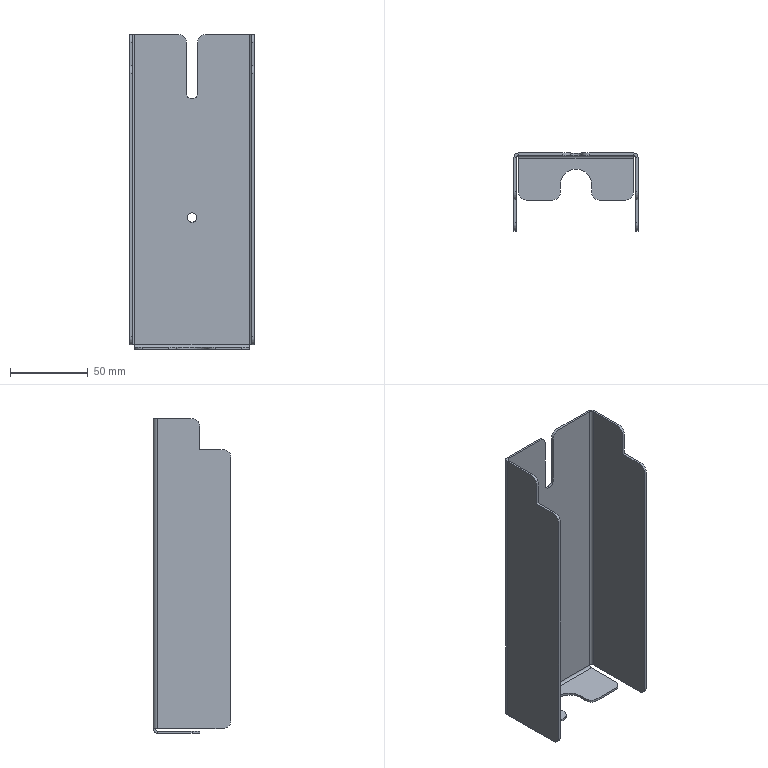Part | NX | features BREP 1 | 1 solid | 55 faces | box 80 x 50 x 203 mm | volume 53607 mm3 | plane 34 | cylinder 21 | commonest cylinder face diameters 10 x12 6 x4 3 x3 7 x1 20 x1
STEP:
#1=CARTESIAN_POINT('',(32.,-30.,-1.5));
#2=VERTEX_POINT('',#1);
#3=CARTESIAN_POINT('',(15.,-30.,-1.5));
#4=VERTEX_POINT('',#3);
#5=CARTESIAN_POINT('',(-37.,-30.,-1.5));
#6=DIRECTION('',(-1.,0.,0.));
#7=VECTOR('',#6,1000.);
#8=LINE('',#5,#7);
#9=EDGE_CURVE('',#2,#4,#8,.T.);
#10=ORIENTED_EDGE('',*,*,#9,.T.);
#11=CARTESIAN_POINT('',(15.,-30.,-3.));
#12=VERTEX_POINT('',#11);
#13=CARTESIAN_POINT('',(15.,-30.,-3.));
#14=DIRECTION('',(0.,0.,-1.));
#15=VECTOR('',#14,1000.);
#16=LINE('',#13,#15);
#17=EDGE_CURVE('',#4,#12,#16,.T.);
#18=ORIENTED_EDGE('',*,*,#17,.T.);
#19=CARTESIAN_POINT('',(32.,-30.,-3.));
#20=VERTEX_POINT('',#19);
#21=CARTESIAN_POINT('',(0.,-30.,-3.));
#22=DIRECTION('',(-1.,0.,0.));
#23=VECTOR('',#22,1000.);
#24=LINE('',#21,#23);
#25=EDGE_CURVE('',#20,#12,#24,.T.);
#26=ORIENTED_EDGE('',*,*,#25,.F.);
#27=CARTESIAN_POINT('',(32.,-30.,-3.));
#28=DIRECTION('',(0.,0.,1.));
#29=VECTOR('',#28,1000.);
#30=LINE('',#27,#29);
#31=EDGE_CURVE('',#20,#2,#30,.T.);
#32=ORIENTED_EDGE('',*,*,#31,.T.);
#33=EDGE_LOOP('',(#10,#18,#26,#32));
#34=FACE_BOUND('',#33,.T.);
#35=CARTESIAN_POINT('',(-37.,-30.,-3.));
#36=DIRECTION('',(0.,1.,0.));
#37=DIRECTION('',(0.,0.,-1.));
#38=AXIS2_PLACEMENT_3D('',#35,#36,#37);
#39=PLANE('',#38);
#40=ADVANCED_FACE('',(#34),#39,.F.);
#41=CARTESIAN_POINT('',(-37.,-1.5,200.));
#42=VERTEX_POINT('',#41);
#43=CARTESIAN_POINT('',(-8.5,-1.5,200.));
#44=VERTEX_POINT('',#43);
#45=CARTESIAN_POINT('',(-40.,-1.5,200.));
#46=DIRECTION('',(1.,0.,0.));
#47=VECTOR('',#46,1000.);
#48=LINE('',#45,#47);
#49=EDGE_CURVE('',#42,#44,#48,.T.);
#50=ORIENTED_EDGE('',*,*,#49,.T.);
#51=CARTESIAN_POINT('',(-8.5,0.,200.));
#52=VERTEX_POINT('',#51);
#53=CARTESIAN_POINT('',(-8.5,0.,200.));
#54=DIRECTION('',(0.,1.,0.));
#55=VECTOR('',#54,1000.);
#56=LINE('',#53,#55);
#57=EDGE_CURVE('',#44,#52,#56,.T.);
#58=ORIENTED_EDGE('',*,*,#57,.T.);
#59=CARTESIAN_POINT('',(-37.,0.,200.));
#60=VERTEX_POINT('',#59);
#61=CARTESIAN_POINT('',(-40.,0.,200.));
#62=DIRECTION('',(1.,0.,0.));
#63=VECTOR('',#62,1000.);
#64=LINE('',#61,#63);
#65=EDGE_CURVE('',#60,#52,#64,.T.);
#66=ORIENTED_EDGE('',*,*,#65,.F.);
#67=CARTESIAN_POINT('',(-37.,0.,200.));
#68=DIRECTION('',(0.,-1.,0.));
#69=VECTOR('',#68,1000.);
#70=LINE('',#67,#69);
#71=EDGE_CURVE('',#60,#42,#70,.T.);
#72=ORIENTED_EDGE('',*,*,#71,.T.);
#73=EDGE_LOOP('',(#50,#58,#66,#72));
#74=FACE_BOUND('',#73,.T.);
#75=CARTESIAN_POINT('',(-38.5,-3.,200.));
#76=DIRECTION('',(0.,0.,1.));
#77=DIRECTION('',(-1.,0.,0.));
#78=AXIS2_PLACEMENT_3D('',#75,#76,#77);
#79=PLANE('',#78);
#80=ADVANCED_FACE('',(#74),#79,.T.);
#81=ORIENTED_EDGE('',*,*,#71,.F.);
#82=CARTESIAN_POINT('',(-40.,-3.,200.));
#83=VERTEX_POINT('',#82);
#84=CARTESIAN_POINT('',(-37.,-3.,200.));
#85=DIRECTION('',(0.,0.,-1.));
#86=DIRECTION('',(1.,0.,0.));
#87=AXIS2_PLACEMENT_3D('',#84,#85,#86);
#88=CIRCLE('',#87,3.);
#89=EDGE_CURVE('',#83,#60,#88,.T.);
#90=ORIENTED_EDGE('',*,*,#89,.F.);
#91=CARTESIAN_POINT('',(-38.5,-3.,200.));
#92=VERTEX_POINT('',#91);
#93=CARTESIAN_POINT('',(-38.5,-3.,200.));
#94=DIRECTION('',(-1.,0.,0.));
#95=VECTOR('',#94,1000.);
#96=LINE('',#93,#95);
#97=EDGE_CURVE('',#92,#83,#96,.T.);
#98=ORIENTED_EDGE('',*,*,#97,.F.);
#99=CARTESIAN_POINT('',(-37.,-3.,200.));
#100=DIRECTION('',(0.,0.,-1.));
#101=DIRECTION('',(1.,0.,0.));
#102=AXIS2_PLACEMENT_3D('',#99,#100,#101);
#103=CIRCLE('',#102,1.5);
#104=EDGE_CURVE('',#92,#42,#103,.T.);
#105=ORIENTED_EDGE('',*,*,#104,.T.);
#106=EDGE_LOOP('',(#81,#90,#98,#105));
#107=FACE_BOUND('',#106,.T.);
#108=CARTESIAN_POINT('',(-37.,0.,200.));
#109=DIRECTION('',(0.,0.,1.));
#110=DIRECTION('',(-1.,0.,0.));
#111=AXIS2_PLACEMENT_3D('',#108,#109,#110);
#112=PLANE('',#111);
#113=ADVANCED_FACE('',(#107),#112,.T.);
#114=CARTESIAN_POINT('',(8.5,0.,200.));
#115=VERTEX_POINT('',#114);
#116=CARTESIAN_POINT('',(37.,0.,200.));
#117=VERTEX_POINT('',#116);
#118=CARTESIAN_POINT('',(-40.,0.,200.));
#119=DIRECTION('',(1.,0.,0.));
#120=VECTOR('',#119,1000.);
#121=LINE('',#118,#120);
#122=EDGE_CURVE('',#115,#117,#121,.T.);
#123=ORIENTED_EDGE('',*,*,#122,.F.);
#124=CARTESIAN_POINT('',(8.5,-1.5,200.));
#125=VERTEX_POINT('',#124);
#126=CARTESIAN_POINT('',(8.5,-1.5,200.));
#127=DIRECTION('',(0.,-1.,0.));
#128=VECTOR('',#127,1000.);
#129=LINE('',#126,#128);
#130=EDGE_CURVE('',#115,#125,#129,.T.);
#131=ORIENTED_EDGE('',*,*,#130,.T.);
#132=CARTESIAN_POINT('',(37.,-1.5,200.));
#133=VERTEX_POINT('',#132);
#134=CARTESIAN_POINT('',(-40.,-1.5,200.));
#135=DIRECTION('',(1.,0.,0.));
#136=VECTOR('',#135,1000.);
#137=LINE('',#134,#136);
#138=EDGE_CURVE('',#125,#133,#137,.T.);
#139=ORIENTED_EDGE('',*,*,#138,.T.);
#140=CARTESIAN_POINT('',(37.,-1.5,200.));
#141=DIRECTION('',(0.,1.,0.));
#142=VECTOR('',#141,1000.);
#143=LINE('',#140,#142);
#144=EDGE_CURVE('',#133,#117,#143,.T.);
#145=ORIENTED_EDGE('',*,*,#144,.T.);
#146=EDGE_LOOP('',(#123,#131,#139,#145));
#147=FACE_BOUND('',#146,.T.);
#148=CARTESIAN_POINT('',(-38.5,-3.,200.));
#149=DIRECTION('',(0.,0.,1.));
#150=DIRECTION('',(-1.,0.,0.));
#151=AXIS2_PLACEMENT_3D('',#148,#149,#150);
#152=PLANE('',#151);
#153=ADVANCED_FACE('',(#147),#152,.T.);
#154=CARTESIAN_POINT('',(-40.,-3.,0.));
#155=VERTEX_POINT('',#154);
#156=CARTESIAN_POINT('',(-38.5,-3.,0.));
#157=VERTEX_POINT('',#156);
#158=CARTESIAN_POINT('',(-40.,-3.,0.));
#159=DIRECTION('',(1.,0.,0.));
#160=VECTOR('',#159,1000.);
#161=LINE('',#158,#160);
#162=EDGE_CURVE('',#155,#157,#161,.T.);
#163=ORIENTED_EDGE('',*,*,#162,.F.);
#164=CARTESIAN_POINT('',(-37.,0.,0.));
#165=VERTEX_POINT('',#164);
#166=CARTESIAN_POINT('',(-37.,-3.,0.));
#167=DIRECTION('',(0.,0.,-1.));
#168=DIRECTION('',(1.,0.,0.));
#169=AXIS2_PLACEMENT_3D('',#166,#167,#168);
#170=CIRCLE('',#169,3.);
#171=EDGE_CURVE('',#155,#165,#170,.T.);
#172=ORIENTED_EDGE('',*,*,#171,.T.);
#173=CARTESIAN_POINT('',(-37.,-1.5,0.));
#174=VERTEX_POINT('',#173);
#175=CARTESIAN_POINT('',(-37.,-1.5,0.));
#176=DIRECTION('',(0.,1.,0.));
#177=VECTOR('',#176,1000.);
#178=LINE('',#175,#177);
#179=EDGE_CURVE('',#174,#165,#178,.T.);
#180=ORIENTED_EDGE('',*,*,#179,.F.);
#181=CARTESIAN_POINT('',(-37.,-3.,0.));
#182=DIRECTION('',(0.,0.,-1.));
#183=DIRECTION('',(1.,0.,0.));
#184=AXIS2_PLACEMENT_3D('',#181,#182,#183);
#185=CIRCLE('',#184,1.5);
#186=EDGE_CURVE('',#157,#174,#185,.T.);
#187=ORIENTED_EDGE('',*,*,#186,.F.);
#188=EDGE_LOOP('',(#163,#172,#180,#187));
#189=FACE_BOUND('',#188,.T.);
#190=CARTESIAN_POINT('',(-40.,-3.,0.));
#191=DIRECTION('',(0.,0.,-1.));
#192=DIRECTION('',(1.,0.,0.));
#193=AXIS2_PLACEMENT_3D('',#190,#191,#192);
#194=PLANE('',#193);
#195=ADVANCED_FACE('',(#189),#194,.T.);
#196=CARTESIAN_POINT('',(-38.5,-45.,0.));
#197=VERTEX_POINT('',#196);
#198=CARTESIAN_POINT('',(-38.5,-50.,0.));
#199=DIRECTION('',(0.,1.,0.));
#200=VECTOR('',#199,1000.);
#201=LINE('',#198,#200);
#202=EDGE_CURVE('',#197,#157,#201,.T.);
#203=ORIENTED_EDGE('',*,*,#202,.F.);
#204=CARTESIAN_POINT('',(-40.,-45.,0.));
#205=VERTEX_POINT('',#204);
#206=CARTESIAN_POINT('',(-37.,-45.,0.));
#207=DIRECTION('',(-1.,0.,0.));
#208=VECTOR('',#207,1000.);
#209=LINE('',#206,#208);
#210=EDGE_CURVE('',#197,#205,#209,.T.);
#211=ORIENTED_EDGE('',*,*,#210,.T.);
#212=CARTESIAN_POINT('',(-40.,-50.,0.));
#213=DIRECTION('',(0.,1.,0.));
#214=VECTOR('',#213,1000.);
#215=LINE('',#212,#214);
#216=EDGE_CURVE('',#205,#155,#215,.T.);
#217=ORIENTED_EDGE('',*,*,#216,.T.);
#218=ORIENTED_EDGE('',*,*,#162,.T.);
#219=EDGE_LOOP('',(#203,#211,#217,#218));
#220=FACE_BOUND('',#219,.T.);
#221=CARTESIAN_POINT('',(-37.,-1.5,0.));
#222=DIRECTION('',(0.,0.,-1.));
#223=DIRECTION('',(1.,0.,0.));
#224=AXIS2_PLACEMENT_3D('',#221,#222,#223);
#225=PLANE('',#224);
#226=ADVANCED_FACE('',(#220),#225,.T.);
#227=CARTESIAN_POINT('',(40.,-3.,200.));
#228=VERTEX_POINT('',#227);
#229=CARTESIAN_POINT('',(38.5,-3.,200.));
#230=VERTEX_POINT('',#229);
#231=CARTESIAN_POINT('',(40.,-3.,200.));
#232=DIRECTION('',(-1.,0.,0.));
#233=VECTOR('',#232,1000.);
#234=LINE('',#231,#233);
#235=EDGE_CURVE('',#228,#230,#234,.T.);
#236=ORIENTED_EDGE('',*,*,#235,.F.);
#237=CARTESIAN_POINT('',(37.,-3.,200.));
#238=DIRECTION('',(0.,0.,-1.));
#239=DIRECTION('',(1.,0.,0.));
#240=AXIS2_PLACEMENT_3D('',#237,#238,#239);
#241=CIRCLE('',#240,3.);
#242=EDGE_CURVE('',#117,#228,#241,.T.);
#243=ORIENTED_EDGE('',*,*,#242,.F.);
#244=ORIENTED_EDGE('',*,*,#144,.F.);
#245=CARTESIAN_POINT('',(37.,-3.,200.));
#246=DIRECTION('',(0.,0.,-1.));
#247=DIRECTION('',(1.,0.,0.));
#248=AXIS2_PLACEMENT_3D('',#245,#246,#247);
#249=CIRCLE('',#248,1.5);
#250=EDGE_CURVE('',#133,#230,#249,.T.);
#251=ORIENTED_EDGE('',*,*,#250,.T.);
#252=EDGE_LOOP('',(#236,#243,#244,#251));
#253=FACE_BOUND('',#252,.T.);
#254=CARTESIAN_POINT('',(40.,-3.,200.));
#255=DIRECTION('',(0.,0.,1.));
#256=DIRECTION('',(-1.,0.,0.));
#257=AXIS2_PLACEMENT_3D('',#254,#255,#256);
#258=PLANE('',#257);
#259=ADVANCED_FACE('',(#253),#258,.T.);
#260=CARTESIAN_POINT('',(38.5,-25.,200.));
#261=VERTEX_POINT('',#260);
#262=CARTESIAN_POINT('',(38.5,0.,200.));
#263=DIRECTION('',(0.,-1.,0.));
#264=VECTOR('',#263,1000.);
#265=LINE('',#262,#264);
#266=EDGE_CURVE('',#230,#261,#265,.T.);
#267=ORIENTED_EDGE('',*,*,#266,.T.);
#268=CARTESIAN_POINT('',(40.,-25.,200.));
#269=VERTEX_POINT('',#268);
#270=CARTESIAN_POINT('',(40.,-25.,200.));
#271=DIRECTION('',(1.,0.,0.));
#272=VECTOR('',#271,1000.);
#273=LINE('',#270,#272);
#274=EDGE_CURVE('',#261,#269,#273,.T.);
#275=ORIENTED_EDGE('',*,*,#274,.T.);
#276=CARTESIAN_POINT('',(40.,0.,200.));
#277=DIRECTION('',(0.,-1.,0.));
#278=VECTOR('',#277,1000.);
#279=LINE('',#276,#278);
#280=EDGE_CURVE('',#228,#269,#279,.T.);
#281=ORIENTED_EDGE('',*,*,#280,.F.);
#282=ORIENTED_EDGE('',*,*,#235,.T.);
#283=EDGE_LOOP('',(#267,#275,#281,#282));
#284=FACE_BOUND('',#283,.T.);
#285=CARTESIAN_POINT('',(37.,-1.5,200.));
#286=DIRECTION('',(0.,0.,1.));
#287=DIRECTION('',(-1.,0.,0.));
#288=AXIS2_PLACEMENT_3D('',#285,#286,#287);
#289=PLANE('',#288);
#290=ADVANCED_FACE('',(#284),#289,.T.);
#291=CARTESIAN_POINT('',(37.,0.,0.));
#292=VERTEX_POINT('',#291);
#293=CARTESIAN_POINT('',(37.,-1.5,0.));
#294=VERTEX_POINT('',#293);
#295=CARTESIAN_POINT('',(37.,0.,0.));
#296=DIRECTION('',(0.,-1.,0.));
#297=VECTOR('',#296,1000.);
#298=LINE('',#295,#297);
#299=EDGE_CURVE('',#292,#294,#298,.T.);
#300=ORIENTED_EDGE('',*,*,#299,.F.);
#301=CARTESIAN_POINT('',(40.,-3.,0.));
#302=VERTEX_POINT('',#301);
#303=CARTESIAN_POINT('',(37.,-3.,0.));
#304=DIRECTION('',(0.,0.,-1.));
#305=DIRECTION('',(1.,0.,0.));
#306=AXIS2_PLACEMENT_3D('',#303,#304,#305);
#307=CIRCLE('',#306,3.);
#308=EDGE_CURVE('',#292,#302,#307,.T.);
#309=ORIENTED_EDGE('',*,*,#308,.T.);
#310=CARTESIAN_POINT('',(38.5,-3.,0.));
#311=VERTEX_POINT('',#310);
#312=CARTESIAN_POINT('',(38.5,-3.,0.));
#313=DIRECTION('',(1.,0.,0.));
#314=VECTOR('',#313,1000.);
#315=LINE('',#312,#314);
#316=EDGE_CURVE('',#311,#302,#315,.T.);
#317=ORIENTED_EDGE('',*,*,#316,.F.);
#318=CARTESIAN_POINT('',(37.,-3.,0.));
#319=DIRECTION('',(0.,0.,-1.));
#320=DIRECTION('',(1.,0.,0.));
#321=AXIS2_PLACEMENT_3D('',#318,#319,#320);
#322=CIRCLE('',#321,1.5);
#323=EDGE_CURVE('',#294,#311,#322,.T.);
#324=ORIENTED_EDGE('',*,*,#323,.F.);
#325=EDGE_LOOP('',(#300,#309,#317,#324));
#326=FACE_BOUND('',#325,.T.);
#327=CARTESIAN_POINT('',(37.,0.,0.));
#328=DIRECTION('',(0.,0.,-1.));
#329=DIRECTION('',(1.,0.,0.));
#330=AXIS2_PLACEMENT_3D('',#327,#328,#329);
#331=PLANE('',#330);
#332=ADVANCED_FACE('',(#326),#331,.T.);
#333=CARTESIAN_POINT('',(38.5,-45.,0.));
#334=VERTEX_POINT('',#333);
#335=CARTESIAN_POINT('',(38.5,0.,0.));
#336=DIRECTION('',(0.,-1.,0.));
#337=VECTOR('',#336,1000.);
#338=LINE('',#335,#337);
#339=EDGE_CURVE('',#311,#334,#338,.T.);
#340=ORIENTED_EDGE('',*,*,#339,.T.);
#341=CARTESIAN_POINT('',(38.5,-50.,5.));
#342=VERTEX_POINT('',#341);
#343=CARTESIAN_POINT('',(38.5,-45.,5.));
#344=DIRECTION('',(-1.,0.,0.));
#345=DIRECTION('',(0.,1.,0.));
#346=AXIS2_PLACEMENT_3D('',#343,#344,#345);
#347=CIRCLE('',#346,5.);
#348=EDGE_CURVE('',#334,#342,#347,.T.);
#349=ORIENTED_EDGE('',*,*,#348,.T.);
#350=CARTESIAN_POINT('',(38.5,-50.,175.));
#351=VERTEX_POINT('',#350);
#352=CARTESIAN_POINT('',(38.5,-50.,200.));
#353=DIRECTION('',(0.,0.,-1.));
#354=VECTOR('',#353,1000.);
#355=LINE('',#352,#354);
#356=EDGE_CURVE('',#351,#342,#355,.T.);
#357=ORIENTED_EDGE('',*,*,#356,.F.);
#358=CARTESIAN_POINT('',(38.5,-45.,180.));
#359=VERTEX_POINT('',#358);
#360=CARTESIAN_POINT('',(38.5,-45.,175.));
#361=DIRECTION('',(-1.,0.,0.));
#362=DIRECTION('',(0.,1.,0.));
#363=AXIS2_PLACEMENT_3D('',#360,#361,#362);
#364=CIRCLE('',#363,5.);
#365=EDGE_CURVE('',#351,#359,#364,.T.);
#366=ORIENTED_EDGE('',*,*,#365,.T.);
#367=CARTESIAN_POINT('',(38.5,-30.,180.));
#368=VERTEX_POINT('',#367);
#369=CARTESIAN_POINT('',(38.5,0.,180.));
#370=DIRECTION('',(0.,1.,0.));
#371=VECTOR('',#370,1000.);
#372=LINE('',#369,#371);
#373=EDGE_CURVE('',#359,#368,#372,.T.);
#374=ORIENTED_EDGE('',*,*,#373,.T.);
#375=CARTESIAN_POINT('',(38.5,-30.,195.));
#376=VERTEX_POINT('',#375);
#377=CARTESIAN_POINT('',(38.5,-30.,200.));
#378=DIRECTION('',(0.,0.,1.));
#379=VECTOR('',#378,1000.);
#380=LINE('',#377,#379);
#381=EDGE_CURVE('',#368,#376,#380,.T.);
#382=ORIENTED_EDGE('',*,*,#381,.T.);
#383=CARTESIAN_POINT('',(38.5,-25.,195.));
#384=DIRECTION('',(-1.,0.,0.));
#385=DIRECTION('',(0.,1.,0.));
#386=AXIS2_PLACEMENT_3D('',#383,#384,#385);
#387=CIRCLE('',#386,5.);
#388=EDGE_CURVE('',#376,#261,#387,.T.);
#389=ORIENTED_EDGE('',*,*,#388,.T.);
#390=ORIENTED_EDGE('',*,*,#266,.F.);
#391=CARTESIAN_POINT('',(38.5,-3.,200.));
#392=DIRECTION('',(0.,0.,-1.));
#393=VECTOR('',#392,1000.);
#394=LINE('',#391,#393);
#395=EDGE_CURVE('',#230,#311,#394,.T.);
#396=ORIENTED_EDGE('',*,*,#395,.T.);
#397=EDGE_LOOP('',(#340,#349,#357,#366,#374,#382,#389,#390,#396));
#398=FACE_BOUND('',#397,.T.);
#399=CARTESIAN_POINT('',(38.5,0.,200.));
#400=DIRECTION('',(1.,0.,0.));
#401=DIRECTION('',(0.,-1.,0.));
#402=AXIS2_PLACEMENT_3D('',#399,#400,#401);
#403=PLANE('',#402);
#404=ADVANCED_FACE('',(#398),#403,.F.);
#405=ORIENTED_EDGE('',*,*,#356,.T.);
#406=CARTESIAN_POINT('',(40.,-50.,5.));
#407=VERTEX_POINT('',#406);
#408=CARTESIAN_POINT('',(40.,-50.,5.));
#409=DIRECTION('',(1.,0.,0.));
#410=VECTOR('',#409,1000.);
#411=LINE('',#408,#410);
#412=EDGE_CURVE('',#342,#407,#411,.T.);
#413=ORIENTED_EDGE('',*,*,#412,.T.);
#414=CARTESIAN_POINT('',(40.,-50.,175.));
#415=VERTEX_POINT('',#414);
#416=CARTESIAN_POINT('',(40.,-50.,200.));
#417=DIRECTION('',(0.,0.,-1.));
#418=VECTOR('',#417,1000.);
#419=LINE('',#416,#418);
#420=EDGE_CURVE('',#415,#407,#419,.T.);
#421=ORIENTED_EDGE('',*,*,#420,.F.);
#422=CARTESIAN_POINT('',(38.5,-50.,175.));
#423=DIRECTION('',(-1.,0.,0.));
#424=VECTOR('',#423,1000.);
#425=LINE('',#422,#424);
#426=EDGE_CURVE('',#415,#351,#425,.T.);
#427=ORIENTED_EDGE('',*,*,#426,.T.);
#428=EDGE_LOOP('',(#405,#413,#421,#427));
#429=FACE_BOUND('',#428,.T.);
#430=CARTESIAN_POINT('',(40.,-50.,200.));
#431=DIRECTION('',(0.,-1.,0.));
#432=DIRECTION('',(0.,0.,1.));
#433=AXIS2_PLACEMENT_3D('',#430,#431,#432);
#434=PLANE('',#433);
#435=ADVANCED_FACE('',(#429),#434,.T.);
#436=ORIENTED_EDGE('',*,*,#420,.T.);
#437=CARTESIAN_POINT('',(40.,-45.,0.));
#438=VERTEX_POINT('',#437);
#439=CARTESIAN_POINT('',(40.,-45.,5.));
#440=DIRECTION('',(1.,0.,0.));
#441=DIRECTION('',(0.,1.,0.));
#442=AXIS2_PLACEMENT_3D('',#439,#440,#441);
#443=CIRCLE('',#442,5.);
#444=EDGE_CURVE('',#407,#438,#443,.T.);
#445=ORIENTED_EDGE('',*,*,#444,.T.);
#446=CARTESIAN_POINT('',(40.,0.,0.));
#447=DIRECTION('',(0.,-1.,0.));
#448=VECTOR('',#447,1000.);
#449=LINE('',#446,#448);
#450=EDGE_CURVE('',#302,#438,#449,.T.);
#451=ORIENTED_EDGE('',*,*,#450,.F.);
#452=CARTESIAN_POINT('',(40.,-3.,200.));
#453=DIRECTION('',(0.,0.,-1.));
#454=VECTOR('',#453,1000.);
#455=LINE('',#452,#454);
#456=EDGE_CURVE('',#228,#302,#455,.T.);
#457=ORIENTED_EDGE('',*,*,#456,.F.);
#458=ORIENTED_EDGE('',*,*,#280,.T.);
#459=CARTESIAN_POINT('',(40.,-30.,195.));
#460=VERTEX_POINT('',#459);
#461=CARTESIAN_POINT('',(40.,-25.,195.));
#462=DIRECTION('',(1.,0.,0.));
#463=DIRECTION('',(0.,1.,0.));
#464=AXIS2_PLACEMENT_3D('',#461,#462,#463);
#465=CIRCLE('',#464,5.);
#466=EDGE_CURVE('',#269,#460,#465,.T.);
#467=ORIENTED_EDGE('',*,*,#466,.T.);
#468=CARTESIAN_POINT('',(40.,-30.,180.));
#469=VERTEX_POINT('',#468);
#470=CARTESIAN_POINT('',(40.,-30.,200.));
#471=DIRECTION('',(0.,0.,1.));
#472=VECTOR('',#471,1000.);
#473=LINE('',#470,#472);
#474=EDGE_CURVE('',#469,#460,#473,.T.);
#475=ORIENTED_EDGE('',*,*,#474,.F.);
#476=CARTESIAN_POINT('',(40.,-45.,180.));
#477=VERTEX_POINT('',#476);
#478=CARTESIAN_POINT('',(40.,-30.,180.));
#479=DIRECTION('',(0.,1.,0.));
#480=VECTOR('',#479,1000.);
#481=LINE('',#478,#480);
#482=EDGE_CURVE('',#477,#469,#481,.T.);
#483=ORIENTED_EDGE('',*,*,#482,.F.);
#484=CARTESIAN_POINT('',(40.,-45.,175.));
#485=DIRECTION('',(1.,0.,0.));
#486=DIRECTION('',(0.,1.,0.));
#487=AXIS2_PLACEMENT_3D('',#484,#485,#486);
#488=CIRCLE('',#487,5.);
#489=EDGE_CURVE('',#477,#415,#488,.T.);
#490=ORIENTED_EDGE('',*,*,#489,.T.);
#491=EDGE_LOOP('',(#436,#445,#451,#457,#458,#467,#475,#483,#490));
#492=FACE_BOUND('',#491,.T.);
#493=CARTESIAN_POINT('',(40.,0.,200.));
#494=DIRECTION('',(1.,0.,0.));
#495=DIRECTION('',(0.,-1.,0.));
#496=AXIS2_PLACEMENT_3D('',#493,#494,#495);
#497=PLANE('',#496);
#498=ADVANCED_FACE('',(#492),#497,.T.);
#499=ORIENTED_EDGE('',*,*,#308,.F.);
#500=CARTESIAN_POINT('',(37.,0.,200.));
#501=DIRECTION('',(0.,0.,-1.));
#502=VECTOR('',#501,1000.);
#503=LINE('',#500,#502);
#504=EDGE_CURVE('',#117,#292,#503,.T.);
#505=ORIENTED_EDGE('',*,*,#504,.F.);
#506=ORIENTED_EDGE('',*,*,#242,.T.);
#507=ORIENTED_EDGE('',*,*,#456,.T.);
#508=EDGE_LOOP('',(#499,#505,#506,#507));
#509=FACE_BOUND('',#508,.T.);
#510=CARTESIAN_POINT('',(37.,-3.,200.));
#511=DIRECTION('',(0.,0.,-1.));
#512=DIRECTION('',(1.,0.,0.));
#513=AXIS2_PLACEMENT_3D('',#510,#511,#512);
#514=CYLINDRICAL_SURFACE('',#513,3.);
#515=ADVANCED_FACE('',(#509),#514,.T.);
#516=CARTESIAN_POINT('',(3.5,0.,195.));
#517=VERTEX_POINT('',#516);
#518=CARTESIAN_POINT('',(3.5,0.,162.));
#519=VERTEX_POINT('',#518);
#520=CARTESIAN_POINT('',(3.5,0.,200.));
#521=DIRECTION('',(0.,0.,-1.));
#522=VECTOR('',#521,1000.);
#523=LINE('',#520,#522);
#524=EDGE_CURVE('',#517,#519,#523,.T.);
#525=ORIENTED_EDGE('',*,*,#524,.F.);
#526=CARTESIAN_POINT('',(8.5,0.,195.));
#527=DIRECTION('',(0.,1.,0.));
#528=DIRECTION('',(-1.,0.,0.));
#529=AXIS2_PLACEMENT_3D('',#526,#527,#528);
#530=CIRCLE('',#529,5.);
#531=EDGE_CURVE('',#517,#115,#530,.T.);
#532=ORIENTED_EDGE('',*,*,#531,.T.);
#533=ORIENTED_EDGE('',*,*,#122,.T.);
#534=ORIENTED_EDGE('',*,*,#504,.T.);
#535=CARTESIAN_POINT('',(-40.,0.,0.));
#536=DIRECTION('',(1.,0.,0.));
#537=VECTOR('',#536,1000.);
#538=LINE('',#535,#537);
#539=EDGE_CURVE('',#165,#292,#538,.T.);
#540=ORIENTED_EDGE('',*,*,#539,.F.);
#541=CARTESIAN_POINT('',(-37.,0.,200.));
#542=DIRECTION('',(0.,0.,-1.));
#543=VECTOR('',#542,1000.);
#544=LINE('',#541,#543);
#545=EDGE_CURVE('',#60,#165,#544,.T.);
#546=ORIENTED_EDGE('',*,*,#545,.F.);
#547=ORIENTED_EDGE('',*,*,#65,.T.);
#548=CARTESIAN_POINT('',(-3.5,0.,195.));
#549=VERTEX_POINT('',#548);
#550=CARTESIAN_POINT('',(-8.5,0.,195.));
#551=DIRECTION('',(0.,1.,0.));
#552=DIRECTION('',(-1.,0.,0.));
#553=AXIS2_PLACEMENT_3D('',#550,#551,#552);
#554=CIRCLE('',#553,5.);
#555=EDGE_CURVE('',#52,#549,#554,.T.);
#556=ORIENTED_EDGE('',*,*,#555,.T.);
#557=CARTESIAN_POINT('',(-3.5,0.,162.));
#558=VERTEX_POINT('',#557);
#559=CARTESIAN_POINT('',(-3.5,0.,200.));
#560=DIRECTION('',(0.,0.,1.));
#561=VECTOR('',#560,1000.);
#562=LINE('',#559,#561);
#563=EDGE_CURVE('',#558,#549,#562,.T.);
#564=ORIENTED_EDGE('',*,*,#563,.F.);
#565=CARTESIAN_POINT('',(0.,0.,162.));
#566=DIRECTION('',(0.,1.,0.));
#567=DIRECTION('',(-1.,0.,0.));
#568=AXIS2_PLACEMENT_3D('',#565,#566,#567);
#569=CIRCLE('',#568,3.5);
#570=EDGE_CURVE('',#519,#558,#569,.T.);
#571=ORIENTED_EDGE('',*,*,#570,.F.);
#572=EDGE_LOOP('',(#525,#532,#533,#534,#540,#546,#547,#556,#564,#571));
#573=FACE_BOUND('',#572,.T.);
#574=CARTESIAN_POINT('',(-3.,0.,82.));
#575=VERTEX_POINT('',#574);
#576=CARTESIAN_POINT('',(0.,0.,82.));
#577=DIRECTION('',(0.,1.,0.));
#578=DIRECTION('',(-1.,0.,0.));
#579=AXIS2_PLACEMENT_3D('',#576,#577,#578);
#580=CIRCLE('',#579,3.);
#581=EDGE_CURVE('',#575,#575,#580,.T.);
#582=ORIENTED_EDGE('',*,*,#581,.F.);
#583=EDGE_LOOP('',(#582));
#584=FACE_BOUND('',#583,.T.);
#585=CARTESIAN_POINT('',(-40.,0.,200.));
#586=DIRECTION('',(0.,1.,0.));
#587=DIRECTION('',(1.,0.,0.));
#588=AXIS2_PLACEMENT_3D('',#585,#586,#587);
#589=PLANE('',#588);
#590=ADVANCED_FACE('',(#573,#584),#589,.T.);
#591=ORIENTED_EDGE('',*,*,#171,.F.);
#592=CARTESIAN_POINT('',(-40.,-3.,200.));
#593=DIRECTION('',(0.,0.,-1.));
#594=VECTOR('',#593,1000.);
#595=LINE('',#592,#594);
#596=EDGE_CURVE('',#83,#155,#595,.T.);
#597=ORIENTED_EDGE('',*,*,#596,.F.);
#598=ORIENTED_EDGE('',*,*,#89,.T.);
#599=ORIENTED_EDGE('',*,*,#545,.T.);
#600=EDGE_LOOP('',(#591,#597,#598,#599));
#601=FACE_BOUND('',#600,.T.);
#602=CARTESIAN_POINT('',(-37.,-3.,200.));
#603=DIRECTION('',(0.,0.,-1.));
#604=DIRECTION('',(1.,0.,0.));
#605=AXIS2_PLACEMENT_3D('',#602,#603,#604);
#606=CYLINDRICAL_SURFACE('',#605,3.);
#607=ADVANCED_FACE('',(#601),#606,.T.);
#608=ORIENTED_EDGE('',*,*,#216,.F.);
#609=CARTESIAN_POINT('',(-40.,-50.,5.));
#610=VERTEX_POINT('',#609);
#611=CARTESIAN_POINT('',(-40.,-45.,5.));
#612=DIRECTION('',(-1.,0.,0.));
#613=DIRECTION('',(0.,0.,1.));
#614=AXIS2_PLACEMENT_3D('',#611,#612,#613);
#615=CIRCLE('',#614,5.);
#616=EDGE_CURVE('',#205,#610,#615,.T.);
#617=ORIENTED_EDGE('',*,*,#616,.T.);
#618=CARTESIAN_POINT('',(-40.,-50.,175.));
#619=VERTEX_POINT('',#618);
#620=CARTESIAN_POINT('',(-40.,-50.,200.));
#621=DIRECTION('',(0.,0.,-1.));
#622=VECTOR('',#621,1000.);
#623=LINE('',#620,#622);
#624=EDGE_CURVE('',#619,#610,#623,.T.);
#625=ORIENTED_EDGE('',*,*,#624,.F.);
#626=CARTESIAN_POINT('',(-40.,-45.,180.));
#627=VERTEX_POINT('',#626);
#628=CARTESIAN_POINT('',(-40.,-45.,175.));
#629=DIRECTION('',(-1.,0.,0.));
#630=DIRECTION('',(0.,0.,1.));
#631=AXIS2_PLACEMENT_3D('',#628,#629,#630);
#632=CIRCLE('',#631,5.);
#633=EDGE_CURVE('',#619,#627,#632,.T.);
#634=ORIENTED_EDGE('',*,*,#633,.T.);
#635=CARTESIAN_POINT('',(-40.,-30.,180.));
#636=VERTEX_POINT('',#635);
#637=CARTESIAN_POINT('',(-40.,-30.,180.));
#638=DIRECTION('',(0.,1.,0.));
#639=VECTOR('',#638,1000.);
#640=LINE('',#637,#639);
#641=EDGE_CURVE('',#627,#636,#640,.T.);
#642=ORIENTED_EDGE('',*,*,#641,.T.);
#643=CARTESIAN_POINT('',(-40.,-30.,195.));
#644=VERTEX_POINT('',#643);
#645=CARTESIAN_POINT('',(-40.,-30.,200.));
#646=DIRECTION('',(0.,0.,1.));
#647=VECTOR('',#646,1000.);
#648=LINE('',#645,#647);
#649=EDGE_CURVE('',#636,#644,#648,.T.);
#650=ORIENTED_EDGE('',*,*,#649,.T.);
#651=CARTESIAN_POINT('',(-40.,-25.,200.));
#652=VERTEX_POINT('',#651);
#653=CARTESIAN_POINT('',(-40.,-25.,195.));
#654=DIRECTION('',(-1.,0.,0.));
#655=DIRECTION('',(0.,0.,1.));
#656=AXIS2_PLACEMENT_3D('',#653,#654,#655);
#657=CIRCLE('',#656,5.);
#658=EDGE_CURVE('',#644,#652,#657,.T.);
#659=ORIENTED_EDGE('',*,*,#658,.T.);
#660=CARTESIAN_POINT('',(-40.,-50.,200.));
#661=DIRECTION('',(0.,1.,0.));
#662=VECTOR('',#661,1000.);
#663=LINE('',#660,#662);
#664=EDGE_CURVE('',#652,#83,#663,.T.);
#665=ORIENTED_EDGE('',*,*,#664,.T.);
#666=ORIENTED_EDGE('',*,*,#596,.T.);
#667=EDGE_LOOP('',(#608,#617,#625,#634,#642,#650,#659,#665,#666));
#668=FACE_BOUND('',#667,.T.);
#669=CARTESIAN_POINT('',(-40.,-50.,200.));
#670=DIRECTION('',(-1.,0.,0.));
#671=DIRECTION('',(0.,0.,-1.));
#672=AXIS2_PLACEMENT_3D('',#669,#670,#671);
#673=PLANE('',#672);
#674=ADVANCED_FACE('',(#668),#673,.T.);
#675=ORIENTED_EDGE('',*,*,#624,.T.);
#676=CARTESIAN_POINT('',(-38.5,-50.,5.));
#677=VERTEX_POINT('',#676);
#678=CARTESIAN_POINT('',(-38.5,-50.,5.));
#679=DIRECTION('',(1.,0.,0.));
#680=VECTOR('',#679,1000.);
#681=LINE('',#678,#680);
#682=EDGE_CURVE('',#610,#677,#681,.T.);
#683=ORIENTED_EDGE('',*,*,#682,.T.);
#684=CARTESIAN_POINT('',(-38.5,-50.,175.));
#685=VERTEX_POINT('',#684);
#686=CARTESIAN_POINT('',(-38.5,-50.,200.));
#687=DIRECTION('',(0.,0.,-1.));
#688=VECTOR('',#687,1000.);
#689=LINE('',#686,#688);
#690=EDGE_CURVE('',#685,#677,#689,.T.);
#691=ORIENTED_EDGE('',*,*,#690,.F.);
#692=CARTESIAN_POINT('',(-40.,-50.,175.));
#693=DIRECTION('',(-1.,0.,0.));
#694=VECTOR('',#693,1000.);
#695=LINE('',#692,#694);
#696=EDGE_CURVE('',#685,#619,#695,.T.);
#697=ORIENTED_EDGE('',*,*,#696,.T.);
#698=EDGE_LOOP('',(#675,#683,#691,#697));
#699=FACE_BOUND('',#698,.T.);
#700=CARTESIAN_POINT('',(-38.5,-50.,200.));
#701=DIRECTION('',(0.,-1.,0.));
#702=DIRECTION('',(0.,0.,1.));
#703=AXIS2_PLACEMENT_3D('',#700,#701,#702);
#704=PLANE('',#703);
#705=ADVANCED_FACE('',(#699),#704,.T.);
#706=ORIENTED_EDGE('',*,*,#690,.T.);
#707=CARTESIAN_POINT('',(-38.5,-45.,5.));
#708=DIRECTION('',(1.,0.,0.));
#709=DIRECTION('',(0.,0.,1.));
#710=AXIS2_PLACEMENT_3D('',#707,#708,#709);
#711=CIRCLE('',#710,5.);
#712=EDGE_CURVE('',#677,#197,#711,.T.);
#713=ORIENTED_EDGE('',*,*,#712,.T.);
#714=ORIENTED_EDGE('',*,*,#202,.T.);
#715=CARTESIAN_POINT('',(-38.5,-3.,200.));
#716=DIRECTION('',(0.,0.,-1.));
#717=VECTOR('',#716,1000.);
#718=LINE('',#715,#717);
#719=EDGE_CURVE('',#92,#157,#718,.T.);
#720=ORIENTED_EDGE('',*,*,#719,.F.);
#721=CARTESIAN_POINT('',(-38.5,-25.,200.));
#722=VERTEX_POINT('',#721);
#723=CARTESIAN_POINT('',(-38.5,-50.,200.));
#724=DIRECTION('',(0.,1.,0.));
#725=VECTOR('',#724,1000.);
#726=LINE('',#723,#725);
#727=EDGE_CURVE('',#722,#92,#726,.T.);
#728=ORIENTED_EDGE('',*,*,#727,.F.);
#729=CARTESIAN_POINT('',(-38.5,-30.,195.));
#730=VERTEX_POINT('',#729);
#731=CARTESIAN_POINT('',(-38.5,-25.,195.));
#732=DIRECTION('',(1.,0.,0.));
#733=DIRECTION('',(0.,0.,1.));
#734=AXIS2_PLACEMENT_3D('',#731,#732,#733);
#735=CIRCLE('',#734,5.);
#736=EDGE_CURVE('',#722,#730,#735,.T.);
#737=ORIENTED_EDGE('',*,*,#736,.T.);
#738=CARTESIAN_POINT('',(-38.5,-30.,180.));
#739=VERTEX_POINT('',#738);
#740=CARTESIAN_POINT('',(-38.5,-30.,200.));
#741=DIRECTION('',(0.,0.,-1.));
#742=VECTOR('',#741,1000.);
#743=LINE('',#740,#742);
#744=EDGE_CURVE('',#730,#739,#743,.T.);
#745=ORIENTED_EDGE('',*,*,#744,.T.);
#746=CARTESIAN_POINT('',(-38.5,-45.,180.));
#747=VERTEX_POINT('',#746);
#748=CARTESIAN_POINT('',(-38.5,-50.,180.));
#749=DIRECTION('',(0.,-1.,0.));
#750=VECTOR('',#749,1000.);
#751=LINE('',#748,#750);
#752=EDGE_CURVE('',#739,#747,#751,.T.);
#753=ORIENTED_EDGE('',*,*,#752,.T.);
#754=CARTESIAN_POINT('',(-38.5,-45.,175.));
#755=DIRECTION('',(1.,0.,0.));
#756=DIRECTION('',(0.,0.,1.));
#757=AXIS2_PLACEMENT_3D('',#754,#755,#756);
#758=CIRCLE('',#757,5.);
#759=EDGE_CURVE('',#747,#685,#758,.T.);
#760=ORIENTED_EDGE('',*,*,#759,.T.);
#761=EDGE_LOOP('',(#706,#713,#714,#720,#728,#737,#745,#753,#760));
#762=FACE_BOUND('',#761,.T.);
#763=CARTESIAN_POINT('',(-38.5,-50.,200.));
#764=DIRECTION('',(-1.,0.,0.));
#765=DIRECTION('',(0.,0.,-1.));
#766=AXIS2_PLACEMENT_3D('',#763,#764,#765);
#767=PLANE('',#766);
#768=ADVANCED_FACE('',(#762),#767,.F.);
#769=ORIENTED_EDGE('',*,*,#186,.T.);
#770=CARTESIAN_POINT('',(-37.,-1.5,200.));
#771=DIRECTION('',(0.,0.,-1.));
#772=VECTOR('',#771,1000.);
#773=LINE('',#770,#772);
#774=EDGE_CURVE('',#42,#174,#773,.T.);
#775=ORIENTED_EDGE('',*,*,#774,.F.);
#776=ORIENTED_EDGE('',*,*,#104,.F.);
#777=ORIENTED_EDGE('',*,*,#719,.T.);
#778=EDGE_LOOP('',(#769,#775,#776,#777));
#779=FACE_BOUND('',#778,.T.);
#780=CARTESIAN_POINT('',(-37.,-3.,200.));
#781=DIRECTION('',(0.,0.,-1.));
#782=DIRECTION('',(1.,0.,0.));
#783=AXIS2_PLACEMENT_3D('',#780,#781,#782);
#784=CYLINDRICAL_SURFACE('',#783,1.5);
#785=ADVANCED_FACE('',(#779),#784,.F.);
#786=CARTESIAN_POINT('',(0.,-1.5,79.));
#787=VERTEX_POINT('',#786);
#788=CARTESIAN_POINT('',(0.,-1.5,82.));
#789=DIRECTION('',(0.,-1.,0.));
#790=DIRECTION('',(0.,0.,-1.));
#791=AXIS2_PLACEMENT_3D('',#788,#789,#790);
#792=CIRCLE('',#791,3.);
#793=EDGE_CURVE('',#787,#787,#792,.T.);
#794=ORIENTED_EDGE('',*,*,#793,.F.);
#795=EDGE_LOOP('',(#794));
#796=FACE_BOUND('',#795,.T.);
#797=ORIENTED_EDGE('',*,*,#138,.F.);
#798=CARTESIAN_POINT('',(3.5,-1.5,195.));
#799=VERTEX_POINT('',#798);
#800=CARTESIAN_POINT('',(8.5,-1.5,195.));
#801=DIRECTION('',(0.,-1.,0.));
#802=DIRECTION('',(-1.,0.,0.));
#803=AXIS2_PLACEMENT_3D('',#800,#801,#802);
#804=CIRCLE('',#803,5.);
#805=EDGE_CURVE('',#125,#799,#804,.T.);
#806=ORIENTED_EDGE('',*,*,#805,.T.);
#807=CARTESIAN_POINT('',(3.5,-1.5,162.));
#808=VERTEX_POINT('',#807);
#809=CARTESIAN_POINT('',(3.5,-1.5,200.));
#810=DIRECTION('',(0.,0.,-1.));
#811=VECTOR('',#810,1000.);
#812=LINE('',#809,#811);
#813=EDGE_CURVE('',#799,#808,#812,.T.);
#814=ORIENTED_EDGE('',*,*,#813,.T.);
#815=CARTESIAN_POINT('',(-3.5,-1.5,162.));
#816=VERTEX_POINT('',#815);
#817=CARTESIAN_POINT('',(0.,-1.5,162.));
#818=DIRECTION('',(0.,1.,0.));
#819=DIRECTION('',(-1.,0.,0.));
#820=AXIS2_PLACEMENT_3D('',#817,#818,#819);
#821=CIRCLE('',#820,3.5);
#822=EDGE_CURVE('',#808,#816,#821,.T.);
#823=ORIENTED_EDGE('',*,*,#822,.T.);
#824=CARTESIAN_POINT('',(-3.5,-1.5,195.));
#825=VERTEX_POINT('',#824);
#826=CARTESIAN_POINT('',(-3.5,-1.5,200.));
#827=DIRECTION('',(0.,0.,1.));
#828=VECTOR('',#827,1000.);
#829=LINE('',#826,#828);
#830=EDGE_CURVE('',#816,#825,#829,.T.);
#831=ORIENTED_EDGE('',*,*,#830,.T.);
#832=CARTESIAN_POINT('',(-8.5,-1.5,195.));
#833=DIRECTION('',(0.,-1.,0.));
#834=DIRECTION('',(-1.,0.,0.));
#835=AXIS2_PLACEMENT_3D('',#832,#833,#834);
#836=CIRCLE('',#835,5.);
#837=EDGE_CURVE('',#825,#44,#836,.T.);
#838=ORIENTED_EDGE('',*,*,#837,.T.);
#839=ORIENTED_EDGE('',*,*,#49,.F.);
#840=ORIENTED_EDGE('',*,*,#774,.T.);
#841=CARTESIAN_POINT('',(-40.,-1.5,0.));
#842=DIRECTION('',(1.,0.,0.));
#843=VECTOR('',#842,1000.);
#844=LINE('',#841,#843);
#845=EDGE_CURVE('',#174,#294,#844,.T.);
#846=ORIENTED_EDGE('',*,*,#845,.T.);
#847=CARTESIAN_POINT('',(37.,-1.5,200.));
#848=DIRECTION('',(0.,0.,-1.));
#849=VECTOR('',#848,1000.);
#850=LINE('',#847,#849);
#851=EDGE_CURVE('',#133,#294,#850,.T.);
#852=ORIENTED_EDGE('',*,*,#851,.F.);
#853=EDGE_LOOP('',(#797,#806,#814,#823,#831,#838,#839,#840,#846,#852));
#854=FACE_BOUND('',#853,.T.);
#855=CARTESIAN_POINT('',(-40.,-1.5,200.));
#856=DIRECTION('',(0.,1.,0.));
#857=DIRECTION('',(1.,0.,0.));
#858=AXIS2_PLACEMENT_3D('',#855,#856,#857);
#859=PLANE('',#858);
#860=ADVANCED_FACE('',(#796,#854),#859,.F.);
#861=ORIENTED_EDGE('',*,*,#323,.T.);
#862=ORIENTED_EDGE('',*,*,#395,.F.);
#863=ORIENTED_EDGE('',*,*,#250,.F.);
#864=ORIENTED_EDGE('',*,*,#851,.T.);
#865=EDGE_LOOP('',(#861,#862,#863,#864));
#866=FACE_BOUND('',#865,.T.);
#867=CARTESIAN_POINT('',(37.,-3.,200.));
#868=DIRECTION('',(0.,0.,-1.));
#869=DIRECTION('',(1.,0.,0.));
#870=AXIS2_PLACEMENT_3D('',#867,#868,#869);
#871=CYLINDRICAL_SURFACE('',#870,1.5);
#872=ADVANCED_FACE('',(#866),#871,.F.);
#873=ORIENTED_EDGE('',*,*,#664,.F.);
#874=CARTESIAN_POINT('',(-38.5,-25.,200.));
#875=DIRECTION('',(1.,0.,0.));
#876=VECTOR('',#875,1000.);
#877=LINE('',#874,#876);
#878=EDGE_CURVE('',#652,#722,#877,.T.);
#879=ORIENTED_EDGE('',*,*,#878,.T.);
#880=ORIENTED_EDGE('',*,*,#727,.T.);
#881=ORIENTED_EDGE('',*,*,#97,.T.);
#882=EDGE_LOOP('',(#873,#879,#880,#881));
#883=FACE_BOUND('',#882,.T.);
#884=CARTESIAN_POINT('',(37.,-3.,200.));
#885=DIRECTION('',(0.,0.,1.));
#886=DIRECTION('',(-1.,0.,0.));
#887=AXIS2_PLACEMENT_3D('',#884,#885,#886);
#888=PLANE('',#887);
#889=ADVANCED_FACE('',(#883),#888,.T.);
#890=ORIENTED_EDGE('',*,*,#450,.T.);
#891=CARTESIAN_POINT('',(38.5,-45.,0.));
#892=DIRECTION('',(-1.,0.,0.));
#893=VECTOR('',#892,1000.);
#894=LINE('',#891,#893);
#895=EDGE_CURVE('',#438,#334,#894,.T.);
#896=ORIENTED_EDGE('',*,*,#895,.T.);
#897=ORIENTED_EDGE('',*,*,#339,.F.);
#898=ORIENTED_EDGE('',*,*,#316,.T.);
#899=EDGE_LOOP('',(#890,#896,#897,#898));
#900=FACE_BOUND('',#899,.T.);
#901=CARTESIAN_POINT('',(37.,-3.,0.));
#902=DIRECTION('',(0.,0.,1.));
#903=DIRECTION('',(-1.,0.,0.));
#904=AXIS2_PLACEMENT_3D('',#901,#902,#903);
#905=PLANE('',#904);
#906=ADVANCED_FACE('',(#900),#905,.F.);
#907=CARTESIAN_POINT('',(-37.,-3.,-1.5));
#908=VERTEX_POINT('',#907);
#909=CARTESIAN_POINT('',(-37.,-3.,-3.));
#910=VERTEX_POINT('',#909);
#911=CARTESIAN_POINT('',(-37.,-3.,-3.));
#912=DIRECTION('',(0.,0.,-1.));
#913=VECTOR('',#912,1000.);
#914=LINE('',#911,#913);
#915=EDGE_CURVE('',#908,#910,#914,.T.);
#916=ORIENTED_EDGE('',*,*,#915,.F.);
#917=CARTESIAN_POINT('',(-37.,-3.,0.));
#918=DIRECTION('',(-1.,0.,0.));
#919=DIRECTION('',(0.,1.,0.));
#920=AXIS2_PLACEMENT_3D('',#917,#918,#919);
#921=CIRCLE('',#920,1.5);
#922=EDGE_CURVE('',#174,#908,#921,.T.);
#923=ORIENTED_EDGE('',*,*,#922,.F.);
#924=ORIENTED_EDGE('',*,*,#179,.T.);
#925=CARTESIAN_POINT('',(-37.,-3.,0.));
#926=DIRECTION('',(-1.,0.,0.));
#927=DIRECTION('',(0.,1.,0.));
#928=AXIS2_PLACEMENT_3D('',#925,#926,#927);
#929=CIRCLE('',#928,3.);
#930=EDGE_CURVE('',#165,#910,#929,.T.);
#931=ORIENTED_EDGE('',*,*,#930,.T.);
#932=EDGE_LOOP('',(#916,#923,#924,#931));
#933=FACE_BOUND('',#932,.T.);
#934=CARTESIAN_POINT('',(-37.,-3.,0.));
#935=DIRECTION('',(-1.,0.,0.));
#936=DIRECTION('',(0.,1.,0.));
#937=AXIS2_PLACEMENT_3D('',#934,#935,#936);
#938=PLANE('',#937);
#939=ADVANCED_FACE('',(#933),#938,.T.);
#940=CARTESIAN_POINT('',(37.,-3.,-1.5));
#941=VERTEX_POINT('',#940);
#942=CARTESIAN_POINT('',(37.,-3.,0.));
#943=DIRECTION('',(1.,0.,0.));
#944=DIRECTION('',(0.,1.,0.));
#945=AXIS2_PLACEMENT_3D('',#942,#943,#944);
#946=CIRCLE('',#945,1.5);
#947=EDGE_CURVE('',#941,#294,#946,.T.);
#948=ORIENTED_EDGE('',*,*,#947,.F.);
#949=CARTESIAN_POINT('',(37.,-3.,-3.));
#950=VERTEX_POINT('',#949);
#951=CARTESIAN_POINT('',(37.,-3.,-1.5));
#952=DIRECTION('',(0.,0.,-1.));
#953=VECTOR('',#952,1000.);
#954=LINE('',#951,#953);
#955=EDGE_CURVE('',#941,#950,#954,.T.);
#956=ORIENTED_EDGE('',*,*,#955,.T.);
#957=CARTESIAN_POINT('',(37.,-3.,0.));
#958=DIRECTION('',(1.,0.,0.));
#959=DIRECTION('',(0.,1.,0.));
#960=AXIS2_PLACEMENT_3D('',#957,#958,#959);
#961=CIRCLE('',#960,3.);
#962=EDGE_CURVE('',#950,#292,#961,.T.);
#963=ORIENTED_EDGE('',*,*,#962,.T.);
#964=ORIENTED_EDGE('',*,*,#299,.T.);
#965=EDGE_LOOP('',(#948,#956,#963,#964));
#966=FACE_BOUND('',#965,.T.);
#967=CARTESIAN_POINT('',(37.,-3.,0.));
#968=DIRECTION('',(-1.,0.,0.));
#969=DIRECTION('',(0.,1.,0.));
#970=AXIS2_PLACEMENT_3D('',#967,#968,#969);
#971=PLANE('',#970);
#972=ADVANCED_FACE('',(#966),#971,.F.);
#973=ORIENTED_EDGE('',*,*,#539,.T.);
#974=ORIENTED_EDGE('',*,*,#962,.F.);
#975=CARTESIAN_POINT('',(-37.,-3.,-3.));
#976=DIRECTION('',(-1.,0.,0.));
#977=VECTOR('',#976,1000.);
#978=LINE('',#975,#977);
#979=EDGE_CURVE('',#950,#910,#978,.T.);
#980=ORIENTED_EDGE('',*,*,#979,.T.);
#981=ORIENTED_EDGE('',*,*,#930,.F.);
#982=EDGE_LOOP('',(#973,#974,#980,#981));
#983=FACE_BOUND('',#982,.T.);
#984=CARTESIAN_POINT('',(37.,-3.,0.));
#985=DIRECTION('',(1.,0.,0.));
#986=DIRECTION('',(0.,0.,1.));
#987=AXIS2_PLACEMENT_3D('',#984,#985,#986);
#988=CYLINDRICAL_SURFACE('',#987,3.);
#989=ADVANCED_FACE('',(#983),#988,.T.);
#990=ORIENTED_EDGE('',*,*,#845,.F.);
#991=ORIENTED_EDGE('',*,*,#922,.T.);
#992=CARTESIAN_POINT('',(-37.,-3.,-1.5));
#993=DIRECTION('',(1.,0.,0.));
#994=VECTOR('',#993,1000.);
#995=LINE('',#992,#994);
#996=EDGE_CURVE('',#908,#941,#995,.T.);
#997=ORIENTED_EDGE('',*,*,#996,.T.);
#998=ORIENTED_EDGE('',*,*,#947,.T.);
#999=EDGE_LOOP('',(#990,#991,#997,#998));
#1000=FACE_BOUND('',#999,.T.);
#1001=CARTESIAN_POINT('',(37.,-3.,0.));
#1002=DIRECTION('',(1.,0.,0.));
#1003=DIRECTION('',(0.,0.,1.));
#1004=AXIS2_PLACEMENT_3D('',#1001,#1002,#1003);
#1005=CYLINDRICAL_SURFACE('',#1004,1.5);
#1006=ADVANCED_FACE('',(#1000),#1005,.F.);
#1007=CARTESIAN_POINT('',(-37.,-25.,-3.));
#1008=VERTEX_POINT('',#1007);
#1009=CARTESIAN_POINT('',(-37.,0.,-3.));
#1010=DIRECTION('',(0.,1.,0.));
#1011=VECTOR('',#1010,1000.);
#1012=LINE('',#1009,#1011);
#1013=EDGE_CURVE('',#1008,#910,#1012,.T.);
#1014=ORIENTED_EDGE('',*,*,#1013,.F.);
#1015=CARTESIAN_POINT('',(-37.,-25.,-1.5));
#1016=VERTEX_POINT('',#1015);
#1017=CARTESIAN_POINT('',(-37.,-25.,-3.));
#1018=DIRECTION('',(0.,0.,1.));
#1019=VECTOR('',#1018,1000.);
#1020=LINE('',#1017,#1019);
#1021=EDGE_CURVE('',#1008,#1016,#1020,.T.);
#1022=ORIENTED_EDGE('',*,*,#1021,.T.);
#1023=CARTESIAN_POINT('',(-37.,-1.5,-1.5));
#1024=DIRECTION('',(0.,1.,0.));
#1025=VECTOR('',#1024,1000.);
#1026=LINE('',#1023,#1025);
#1027=EDGE_CURVE('',#1016,#908,#1026,.T.);
#1028=ORIENTED_EDGE('',*,*,#1027,.T.);
#1029=ORIENTED_EDGE('',*,*,#915,.T.);
#1030=EDGE_LOOP('',(#1014,#1022,#1028,#1029));
#1031=FACE_BOUND('',#1030,.T.);
#1032=CARTESIAN_POINT('',(-37.,-1.5,-3.));
#1033=DIRECTION('',(1.,0.,0.));
#1034=DIRECTION('',(0.,-1.,0.));
#1035=AXIS2_PLACEMENT_3D('',#1032,#1033,#1034);
#1036=PLANE('',#1035);
#1037=ADVANCED_FACE('',(#1031),#1036,.F.);
#1038=CARTESIAN_POINT('',(37.,-25.,-1.5));
#1039=VERTEX_POINT('',#1038);
#1040=CARTESIAN_POINT('',(37.,-30.,-1.5));
#1041=DIRECTION('',(0.,-1.,0.));
#1042=VECTOR('',#1041,1000.);
#1043=LINE('',#1040,#1042);
#1044=EDGE_CURVE('',#941,#1039,#1043,.T.);
#1045=ORIENTED_EDGE('',*,*,#1044,.T.);
#1046=CARTESIAN_POINT('',(37.,-25.,-3.));
#1047=VERTEX_POINT('',#1046);
#1048=CARTESIAN_POINT('',(37.,-25.,-3.));
#1049=DIRECTION('',(0.,0.,-1.));
#1050=VECTOR('',#1049,1000.);
#1051=LINE('',#1048,#1050);
#1052=EDGE_CURVE('',#1039,#1047,#1051,.T.);
#1053=ORIENTED_EDGE('',*,*,#1052,.T.);
#1054=CARTESIAN_POINT('',(37.,0.,-3.));
#1055=DIRECTION('',(0.,-1.,0.));
#1056=VECTOR('',#1055,1000.);
#1057=LINE('',#1054,#1056);
#1058=EDGE_CURVE('',#950,#1047,#1057,.T.);
#1059=ORIENTED_EDGE('',*,*,#1058,.F.);
#1060=ORIENTED_EDGE('',*,*,#955,.F.);
#1061=EDGE_LOOP('',(#1045,#1053,#1059,#1060));
#1062=FACE_BOUND('',#1061,.T.);
#1063=CARTESIAN_POINT('',(37.,-30.,-3.));
#1064=DIRECTION('',(-1.,0.,0.));
#1065=DIRECTION('',(0.,1.,0.));
#1066=AXIS2_PLACEMENT_3D('',#1063,#1064,#1065);
#1067=PLANE('',#1066);
#1068=ADVANCED_FACE('',(#1062),#1067,.F.);
#1069=CARTESIAN_POINT('',(-10.,-25.,-3.));
#1070=VERTEX_POINT('',#1069);
#1071=CARTESIAN_POINT('',(-10.,-20.,-3.));
#1072=VERTEX_POINT('',#1071);
#1073=CARTESIAN_POINT('',(-10.,-30.,-3.));
#1074=DIRECTION('',(0.,1.,0.));
#1075=VECTOR('',#1074,1000.);
#1076=LINE('',#1073,#1075);
#1077=EDGE_CURVE('',#1070,#1072,#1076,.T.);
#1078=ORIENTED_EDGE('',*,*,#1077,.F.);
#1079=CARTESIAN_POINT('',(-15.,-30.,-3.));
#1080=VERTEX_POINT('',#1079);
#1081=CARTESIAN_POINT('',(-15.,-25.,-3.));
#1082=DIRECTION('',(0.,0.,-1.));
#1083=DIRECTION('',(0.,-1.,0.));
#1084=AXIS2_PLACEMENT_3D('',#1081,#1082,#1083);
#1085=CIRCLE('',#1084,5.);
#1086=EDGE_CURVE('',#1070,#1080,#1085,.T.);
#1087=ORIENTED_EDGE('',*,*,#1086,.T.);
#1088=CARTESIAN_POINT('',(-32.,-30.,-3.));
#1089=VERTEX_POINT('',#1088);
#1090=CARTESIAN_POINT('',(0.,-30.,-3.));
#1091=DIRECTION('',(-1.,0.,0.));
#1092=VECTOR('',#1091,1000.);
#1093=LINE('',#1090,#1092);
#1094=EDGE_CURVE('',#1080,#1089,#1093,.T.);
#1095=ORIENTED_EDGE('',*,*,#1094,.T.);
#1096=CARTESIAN_POINT('',(-32.,-25.,-3.));
#1097=DIRECTION('',(0.,0.,-1.));
#1098=DIRECTION('',(0.,-1.,0.));
#1099=AXIS2_PLACEMENT_3D('',#1096,#1097,#1098);
#1100=CIRCLE('',#1099,5.);
#1101=EDGE_CURVE('',#1089,#1008,#1100,.T.);
#1102=ORIENTED_EDGE('',*,*,#1101,.T.);
#1103=ORIENTED_EDGE('',*,*,#1013,.T.);
#1104=ORIENTED_EDGE('',*,*,#979,.F.);
#1105=ORIENTED_EDGE('',*,*,#1058,.T.);
#1106=CARTESIAN_POINT('',(32.,-25.,-3.));
#1107=DIRECTION('',(0.,0.,-1.));
#1108=DIRECTION('',(0.,-1.,0.));
#1109=AXIS2_PLACEMENT_3D('',#1106,#1107,#1108);
#1110=CIRCLE('',#1109,5.);
#1111=EDGE_CURVE('',#1047,#20,#1110,.T.);
#1112=ORIENTED_EDGE('',*,*,#1111,.T.);
#1113=ORIENTED_EDGE('',*,*,#25,.T.);
#1114=CARTESIAN_POINT('',(10.,-25.,-3.));
#1115=VERTEX_POINT('',#1114);
#1116=CARTESIAN_POINT('',(15.,-25.,-3.));
#1117=DIRECTION('',(0.,0.,-1.));
#1118=DIRECTION('',(0.,-1.,0.));
#1119=AXIS2_PLACEMENT_3D('',#1116,#1117,#1118);
#1120=CIRCLE('',#1119,5.);
#1121=EDGE_CURVE('',#12,#1115,#1120,.T.);
#1122=ORIENTED_EDGE('',*,*,#1121,.T.);
#1123=CARTESIAN_POINT('',(10.,-20.,-3.));
#1124=VERTEX_POINT('',#1123);
#1125=CARTESIAN_POINT('',(10.,-30.,-3.));
#1126=DIRECTION('',(0.,-1.,0.));
#1127=VECTOR('',#1126,1000.);
#1128=LINE('',#1125,#1127);
#1129=EDGE_CURVE('',#1124,#1115,#1128,.T.);
#1130=ORIENTED_EDGE('',*,*,#1129,.F.);
#1131=CARTESIAN_POINT('',(0.,-20.,-3.));
#1132=DIRECTION('',(0.,0.,-1.));
#1133=DIRECTION('',(0.,1.,0.));
#1134=AXIS2_PLACEMENT_3D('',#1131,#1132,#1133);
#1135=CIRCLE('',#1134,10.);
#1136=EDGE_CURVE('',#1072,#1124,#1135,.T.);
#1137=ORIENTED_EDGE('',*,*,#1136,.F.);
#1138=EDGE_LOOP('',(#1078,#1087,#1095,#1102,#1103,#1104,#1105,#1112,#1113,#1122,#1130,#1137));
#1139=FACE_BOUND('',#1138,.T.);
#1140=CARTESIAN_POINT('',(0.,0.,-3.));
#1141=DIRECTION('',(0.,0.,1.));
#1142=DIRECTION('',(0.,1.,0.));
#1143=AXIS2_PLACEMENT_3D('',#1140,#1141,#1142);
#1144=PLANE('',#1143);
#1145=ADVANCED_FACE('',(#1139),#1144,.F.);
#1146=CARTESIAN_POINT('',(-15.,-30.,-1.5));
#1147=VERTEX_POINT('',#1146);
#1148=CARTESIAN_POINT('',(-32.,-30.,-1.5));
#1149=VERTEX_POINT('',#1148);
#1150=CARTESIAN_POINT('',(-37.,-30.,-1.5));
#1151=DIRECTION('',(-1.,0.,0.));
#1152=VECTOR('',#1151,1000.);
#1153=LINE('',#1150,#1152);
#1154=EDGE_CURVE('',#1147,#1149,#1153,.T.);
#1155=ORIENTED_EDGE('',*,*,#1154,.F.);
#1156=CARTESIAN_POINT('',(-10.,-25.,-1.5));
#1157=VERTEX_POINT('',#1156);
#1158=CARTESIAN_POINT('',(-15.,-25.,-1.5));
#1159=DIRECTION('',(0.,0.,1.));
#1160=DIRECTION('',(0.,-1.,0.));
#1161=AXIS2_PLACEMENT_3D('',#1158,#1159,#1160);
#1162=CIRCLE('',#1161,5.);
#1163=EDGE_CURVE('',#1147,#1157,#1162,.T.);
#1164=ORIENTED_EDGE('',*,*,#1163,.T.);
#1165=CARTESIAN_POINT('',(-10.,-20.,-1.5));
#1166=VERTEX_POINT('',#1165);
#1167=CARTESIAN_POINT('',(-10.,0.,-1.5));
#1168=DIRECTION('',(0.,-1.,0.));
#1169=VECTOR('',#1168,1000.);
#1170=LINE('',#1167,#1169);
#1171=EDGE_CURVE('',#1166,#1157,#1170,.T.);
#1172=ORIENTED_EDGE('',*,*,#1171,.F.);
#1173=CARTESIAN_POINT('',(10.,-20.,-1.5));
#1174=VERTEX_POINT('',#1173);
#1175=CARTESIAN_POINT('',(0.,-20.,-1.5));
#1176=DIRECTION('',(0.,0.,1.));
#1177=DIRECTION('',(0.,-1.,0.));
#1178=AXIS2_PLACEMENT_3D('',#1175,#1176,#1177);
#1179=CIRCLE('',#1178,10.);
#1180=EDGE_CURVE('',#1174,#1166,#1179,.T.);
#1181=ORIENTED_EDGE('',*,*,#1180,.F.);
#1182=CARTESIAN_POINT('',(10.,-25.,-1.5));
#1183=VERTEX_POINT('',#1182);
#1184=CARTESIAN_POINT('',(10.,0.,-1.5));
#1185=DIRECTION('',(0.,1.,0.));
#1186=VECTOR('',#1185,1000.);
#1187=LINE('',#1184,#1186);
#1188=EDGE_CURVE('',#1183,#1174,#1187,.T.);
#1189=ORIENTED_EDGE('',*,*,#1188,.F.);
#1190=CARTESIAN_POINT('',(15.,-25.,-1.5));
#1191=DIRECTION('',(0.,0.,1.));
#1192=DIRECTION('',(0.,-1.,0.));
#1193=AXIS2_PLACEMENT_3D('',#1190,#1191,#1192);
#1194=CIRCLE('',#1193,5.);
#1195=EDGE_CURVE('',#1183,#4,#1194,.T.);
#1196=ORIENTED_EDGE('',*,*,#1195,.T.);
#1197=ORIENTED_EDGE('',*,*,#9,.F.);
#1198=CARTESIAN_POINT('',(32.,-25.,-1.5));
#1199=DIRECTION('',(0.,0.,1.));
#1200=DIRECTION('',(0.,-1.,0.));
#1201=AXIS2_PLACEMENT_3D('',#1198,#1199,#1200);
#1202=CIRCLE('',#1201,5.);
#1203=EDGE_CURVE('',#2,#1039,#1202,.T.);
#1204=ORIENTED_EDGE('',*,*,#1203,.T.);
#1205=ORIENTED_EDGE('',*,*,#1044,.F.);
#1206=ORIENTED_EDGE('',*,*,#996,.F.);
#1207=ORIENTED_EDGE('',*,*,#1027,.F.);
#1208=CARTESIAN_POINT('',(-32.,-25.,-1.5));
#1209=DIRECTION('',(0.,0.,1.));
#1210=DIRECTION('',(0.,-1.,0.));
#1211=AXIS2_PLACEMENT_3D('',#1208,#1209,#1210);
#1212=CIRCLE('',#1211,5.);
#1213=EDGE_CURVE('',#1016,#1149,#1212,.T.);
#1214=ORIENTED_EDGE('',*,*,#1213,.T.);
#1215=EDGE_LOOP('',(#1155,#1164,#1172,#1181,#1189,#1196,#1197,#1204,#1205,#1206,#1207,#1214));
#1216=FACE_BOUND('',#1215,.T.);
#1217=CARTESIAN_POINT('',(0.,0.,-1.5));
#1218=DIRECTION('',(0.,0.,1.));
#1219=DIRECTION('',(0.,1.,0.));
#1220=AXIS2_PLACEMENT_3D('',#1217,#1218,#1219);
#1221=PLANE('',#1220);
#1222=ADVANCED_FACE('',(#1216),#1221,.T.);
#1223=ORIENTED_EDGE('',*,*,#1094,.F.);
#1224=CARTESIAN_POINT('',(-15.,-30.,-3.));
#1225=DIRECTION('',(0.,0.,1.));
#1226=VECTOR('',#1225,1000.);
#1227=LINE('',#1224,#1226);
#1228=EDGE_CURVE('',#1080,#1147,#1227,.T.);
#1229=ORIENTED_EDGE('',*,*,#1228,.T.);
#1230=ORIENTED_EDGE('',*,*,#1154,.T.);
#1231=CARTESIAN_POINT('',(-32.,-30.,-3.));
#1232=DIRECTION('',(0.,0.,-1.));
#1233=VECTOR('',#1232,1000.);
#1234=LINE('',#1231,#1233);
#1235=EDGE_CURVE('',#1149,#1089,#1234,.T.);
#1236=ORIENTED_EDGE('',*,*,#1235,.T.);
#1237=EDGE_LOOP('',(#1223,#1229,#1230,#1236));
#1238=FACE_BOUND('',#1237,.T.);
#1239=CARTESIAN_POINT('',(-37.,-30.,-3.));
#1240=DIRECTION('',(0.,1.,0.));
#1241=DIRECTION('',(0.,0.,-1.));
#1242=AXIS2_PLACEMENT_3D('',#1239,#1240,#1241);
#1243=PLANE('',#1242);
#1244=ADVANCED_FACE('',(#1238),#1243,.F.);
#1245=ORIENTED_EDGE('',*,*,#744,.F.);
#1246=CARTESIAN_POINT('',(-40.,-30.,195.));
#1247=DIRECTION('',(-1.,0.,0.));
#1248=VECTOR('',#1247,1000.);
#1249=LINE('',#1246,#1248);
#1250=EDGE_CURVE('',#730,#644,#1249,.T.);
#1251=ORIENTED_EDGE('',*,*,#1250,.T.);
#1252=ORIENTED_EDGE('',*,*,#649,.F.);
#1253=CARTESIAN_POINT('',(-40.,-30.,180.));
#1254=DIRECTION('',(1.,0.,0.));
#1255=VECTOR('',#1254,1000.);
#1256=LINE('',#1253,#1255);
#1257=EDGE_CURVE('',#636,#739,#1256,.T.);
#1258=ORIENTED_EDGE('',*,*,#1257,.T.);
#1259=EDGE_LOOP('',(#1245,#1251,#1252,#1258));
#1260=FACE_BOUND('',#1259,.T.);
#1261=CARTESIAN_POINT('',(-40.,-30.,200.));
#1262=DIRECTION('',(0.,1.,0.));
#1263=DIRECTION('',(1.,0.,0.));
#1264=AXIS2_PLACEMENT_3D('',#1261,#1262,#1263);
#1265=PLANE('',#1264);
#1266=ADVANCED_FACE('',(#1260),#1265,.F.);
#1267=ORIENTED_EDGE('',*,*,#641,.F.);
#1268=CARTESIAN_POINT('',(-38.5,-45.,180.));
#1269=DIRECTION('',(1.,0.,0.));
#1270=VECTOR('',#1269,1000.);
#1271=LINE('',#1268,#1270);
#1272=EDGE_CURVE('',#627,#747,#1271,.T.);
#1273=ORIENTED_EDGE('',*,*,#1272,.T.);
#1274=ORIENTED_EDGE('',*,*,#752,.F.);
#1275=ORIENTED_EDGE('',*,*,#1257,.F.);
#1276=EDGE_LOOP('',(#1267,#1273,#1274,#1275));
#1277=FACE_BOUND('',#1276,.T.);
#1278=CARTESIAN_POINT('',(-40.,-30.,180.));
#1279=DIRECTION('',(0.,0.,-1.));
#1280=DIRECTION('',(1.,0.,0.));
#1281=AXIS2_PLACEMENT_3D('',#1278,#1279,#1280);
#1282=PLANE('',#1281);
#1283=ADVANCED_FACE('',(#1277),#1282,.F.);
#1284=ORIENTED_EDGE('',*,*,#373,.F.);
#1285=CARTESIAN_POINT('',(40.,-45.,180.));
#1286=DIRECTION('',(1.,0.,0.));
#1287=VECTOR('',#1286,1000.);
#1288=LINE('',#1285,#1287);
#1289=EDGE_CURVE('',#359,#477,#1288,.T.);
#1290=ORIENTED_EDGE('',*,*,#1289,.T.);
#1291=ORIENTED_EDGE('',*,*,#482,.T.);
#1292=CARTESIAN_POINT('',(-40.,-30.,180.));
#1293=DIRECTION('',(1.,0.,0.));
#1294=VECTOR('',#1293,1000.);
#1295=LINE('',#1292,#1294);
#1296=EDGE_CURVE('',#368,#469,#1295,.T.);
#1297=ORIENTED_EDGE('',*,*,#1296,.F.);
#1298=EDGE_LOOP('',(#1284,#1290,#1291,#1297));
#1299=FACE_BOUND('',#1298,.T.);
#1300=CARTESIAN_POINT('',(-40.,-30.,180.));
#1301=DIRECTION('',(0.,0.,-1.));
#1302=DIRECTION('',(1.,0.,0.));
#1303=AXIS2_PLACEMENT_3D('',#1300,#1301,#1302);
#1304=PLANE('',#1303);
#1305=ADVANCED_FACE('',(#1299),#1304,.F.);
#1306=ORIENTED_EDGE('',*,*,#474,.T.);
#1307=CARTESIAN_POINT('',(38.5,-30.,195.));
#1308=DIRECTION('',(-1.,0.,0.));
#1309=VECTOR('',#1308,1000.);
#1310=LINE('',#1307,#1309);
#1311=EDGE_CURVE('',#460,#376,#1310,.T.);
#1312=ORIENTED_EDGE('',*,*,#1311,.T.);
#1313=ORIENTED_EDGE('',*,*,#381,.F.);
#1314=ORIENTED_EDGE('',*,*,#1296,.T.);
#1315=EDGE_LOOP('',(#1306,#1312,#1313,#1314));
#1316=FACE_BOUND('',#1315,.T.);
#1317=CARTESIAN_POINT('',(-40.,-30.,200.));
#1318=DIRECTION('',(0.,1.,0.));
#1319=DIRECTION('',(1.,0.,0.));
#1320=AXIS2_PLACEMENT_3D('',#1317,#1318,#1319);
#1321=PLANE('',#1320);
#1322=ADVANCED_FACE('',(#1316),#1321,.F.);
#1323=ORIENTED_EDGE('',*,*,#581,.T.);
#1324=EDGE_LOOP('',(#1323));
#1325=FACE_BOUND('',#1324,.T.);
#1326=ORIENTED_EDGE('',*,*,#793,.T.);
#1327=EDGE_LOOP('',(#1326));
#1328=FACE_BOUND('',#1327,.T.);
#1329=CARTESIAN_POINT('',(0.,-1.5,82.));
#1330=DIRECTION('',(0.,-1.,0.));
#1331=DIRECTION('',(0.,0.,1.));
#1332=AXIS2_PLACEMENT_3D('',#1329,#1330,#1331);
#1333=CYLINDRICAL_SURFACE('',#1332,3.);
#1334=ADVANCED_FACE('',(#1325,#1328),#1333,.F.);
#1335=ORIENTED_EDGE('',*,*,#563,.T.);
#1336=CARTESIAN_POINT('',(-3.5,-1.5,195.));
#1337=DIRECTION('',(0.,-1.,0.));
#1338=VECTOR('',#1337,1000.);
#1339=LINE('',#1336,#1338);
#1340=EDGE_CURVE('',#549,#825,#1339,.T.);
#1341=ORIENTED_EDGE('',*,*,#1340,.T.);
#1342=ORIENTED_EDGE('',*,*,#830,.F.);
#1343=CARTESIAN_POINT('',(-3.5,-10.,162.));
#1344=DIRECTION('',(0.,1.,0.));
#1345=VECTOR('',#1344,1000.);
#1346=LINE('',#1343,#1345);
#1347=EDGE_CURVE('',#816,#558,#1346,.T.);
#1348=ORIENTED_EDGE('',*,*,#1347,.T.);
#1349=EDGE_LOOP('',(#1335,#1341,#1342,#1348));
#1350=FACE_BOUND('',#1349,.T.);
#1351=CARTESIAN_POINT('',(-3.5,-10.,200.));
#1352=DIRECTION('',(-1.,0.,0.));
#1353=DIRECTION('',(0.,1.,0.));
#1354=AXIS2_PLACEMENT_3D('',#1351,#1352,#1353);
#1355=PLANE('',#1354);
#1356=ADVANCED_FACE('',(#1350),#1355,.F.);
#1357=CARTESIAN_POINT('',(3.5,-10.,162.));
#1358=DIRECTION('',(0.,1.,0.));
#1359=VECTOR('',#1358,1000.);
#1360=LINE('',#1357,#1359);
#1361=EDGE_CURVE('',#808,#519,#1360,.T.);
#1362=ORIENTED_EDGE('',*,*,#1361,.T.);
#1363=ORIENTED_EDGE('',*,*,#570,.T.);
#1364=ORIENTED_EDGE('',*,*,#1347,.F.);
#1365=ORIENTED_EDGE('',*,*,#822,.F.);
#1366=EDGE_LOOP('',(#1362,#1363,#1364,#1365));
#1367=FACE_BOUND('',#1366,.T.);
#1368=CARTESIAN_POINT('',(0.,-10.,162.));
#1369=DIRECTION('',(0.,1.,0.));
#1370=DIRECTION('',(1.,0.,0.));
#1371=AXIS2_PLACEMENT_3D('',#1368,#1369,#1370);
#1372=CYLINDRICAL_SURFACE('',#1371,3.5);
#1373=ADVANCED_FACE('',(#1367),#1372,.F.);
#1374=ORIENTED_EDGE('',*,*,#813,.F.);
#1375=CARTESIAN_POINT('',(3.5,0.,195.));
#1376=DIRECTION('',(0.,1.,0.));
#1377=VECTOR('',#1376,1000.);
#1378=LINE('',#1375,#1377);
#1379=EDGE_CURVE('',#799,#517,#1378,.T.);
#1380=ORIENTED_EDGE('',*,*,#1379,.T.);
#1381=ORIENTED_EDGE('',*,*,#524,.T.);
#1382=ORIENTED_EDGE('',*,*,#1361,.F.);
#1383=EDGE_LOOP('',(#1374,#1380,#1381,#1382));
#1384=FACE_BOUND('',#1383,.T.);
#1385=CARTESIAN_POINT('',(3.5,-10.,200.));
#1386=DIRECTION('',(1.,0.,0.));
#1387=DIRECTION('',(0.,-1.,0.));
#1388=AXIS2_PLACEMENT_3D('',#1385,#1386,#1387);
#1389=PLANE('',#1388);
#1390=ADVANCED_FACE('',(#1384),#1389,.F.);
#1391=ORIENTED_EDGE('',*,*,#1129,.T.);
#1392=CARTESIAN_POINT('',(10.,-25.,7.));
#1393=DIRECTION('',(0.,0.,1.));
#1394=VECTOR('',#1393,1000.);
#1395=LINE('',#1392,#1394);
#1396=EDGE_CURVE('',#1115,#1183,#1395,.T.);
#1397=ORIENTED_EDGE('',*,*,#1396,.T.);
#1398=ORIENTED_EDGE('',*,*,#1188,.T.);
#1399=CARTESIAN_POINT('',(10.,-20.,7.));
#1400=DIRECTION('',(0.,0.,-1.));
#1401=VECTOR('',#1400,1000.);
#1402=LINE('',#1399,#1401);
#1403=EDGE_CURVE('',#1174,#1124,#1402,.T.);
#1404=ORIENTED_EDGE('',*,*,#1403,.T.);
#1405=EDGE_LOOP('',(#1391,#1397,#1398,#1404));
#1406=FACE_BOUND('',#1405,.T.);
#1407=CARTESIAN_POINT('',(10.,-30.,7.));
#1408=DIRECTION('',(1.,0.,0.));
#1409=DIRECTION('',(0.,-1.,0.));
#1410=AXIS2_PLACEMENT_3D('',#1407,#1408,#1409);
#1411=PLANE('',#1410);
#1412=ADVANCED_FACE('',(#1406),#1411,.F.);
#1413=ORIENTED_EDGE('',*,*,#1180,.T.);
#1414=CARTESIAN_POINT('',(-10.,-20.,7.));
#1415=DIRECTION('',(0.,0.,-1.));
#1416=VECTOR('',#1415,1000.);
#1417=LINE('',#1414,#1416);
#1418=EDGE_CURVE('',#1166,#1072,#1417,.T.);
#1419=ORIENTED_EDGE('',*,*,#1418,.T.);
#1420=ORIENTED_EDGE('',*,*,#1136,.T.);
#1421=ORIENTED_EDGE('',*,*,#1403,.F.);
#1422=EDGE_LOOP('',(#1413,#1419,#1420,#1421));
#1423=FACE_BOUND('',#1422,.T.);
#1424=CARTESIAN_POINT('',(0.,-20.,7.));
#1425=DIRECTION('',(0.,0.,-1.));
#1426=DIRECTION('',(0.,-1.,0.));
#1427=AXIS2_PLACEMENT_3D('',#1424,#1425,#1426);
#1428=CYLINDRICAL_SURFACE('',#1427,10.);
#1429=ADVANCED_FACE('',(#1423),#1428,.F.);
#1430=ORIENTED_EDGE('',*,*,#1171,.T.);
#1431=CARTESIAN_POINT('',(-10.,-25.,7.));
#1432=DIRECTION('',(0.,0.,-1.));
#1433=VECTOR('',#1432,1000.);
#1434=LINE('',#1431,#1433);
#1435=EDGE_CURVE('',#1157,#1070,#1434,.T.);
#1436=ORIENTED_EDGE('',*,*,#1435,.T.);
#1437=ORIENTED_EDGE('',*,*,#1077,.T.);
#1438=ORIENTED_EDGE('',*,*,#1418,.F.);
#1439=EDGE_LOOP('',(#1430,#1436,#1437,#1438));
#1440=FACE_BOUND('',#1439,.T.);
#1441=CARTESIAN_POINT('',(-10.,-30.,7.));
#1442=DIRECTION('',(-1.,0.,0.));
#1443=DIRECTION('',(0.,1.,0.));
#1444=AXIS2_PLACEMENT_3D('',#1441,#1442,#1443);
#1445=PLANE('',#1444);
#1446=ADVANCED_FACE('',(#1440),#1445,.F.);
#1447=ORIENTED_EDGE('',*,*,#1086,.F.);
#1448=ORIENTED_EDGE('',*,*,#1435,.F.);
#1449=ORIENTED_EDGE('',*,*,#1163,.F.);
#1450=ORIENTED_EDGE('',*,*,#1228,.F.);
#1451=EDGE_LOOP('',(#1447,#1448,#1449,#1450));
#1452=FACE_BOUND('',#1451,.T.);
#1453=CARTESIAN_POINT('',(-15.,-25.,-3.));
#1454=DIRECTION('',(0.,0.,1.));
#1455=DIRECTION('',(0.,1.,0.));
#1456=AXIS2_PLACEMENT_3D('',#1453,#1454,#1455);
#1457=CYLINDRICAL_SURFACE('',#1456,5.);
#1458=ADVANCED_FACE('',(#1452),#1457,.T.);
#1459=ORIENTED_EDGE('',*,*,#1195,.F.);
#1460=ORIENTED_EDGE('',*,*,#1396,.F.);
#1461=ORIENTED_EDGE('',*,*,#1121,.F.);
#1462=ORIENTED_EDGE('',*,*,#17,.F.);
#1463=EDGE_LOOP('',(#1459,#1460,#1461,#1462));
#1464=FACE_BOUND('',#1463,.T.);
#1465=CARTESIAN_POINT('',(15.,-25.,-3.));
#1466=DIRECTION('',(0.,0.,-1.));
#1467=DIRECTION('',(0.,-1.,0.));
#1468=AXIS2_PLACEMENT_3D('',#1465,#1466,#1467);
#1469=CYLINDRICAL_SURFACE('',#1468,5.);
#1470=ADVANCED_FACE('',(#1464),#1469,.T.);
#1471=ORIENTED_EDGE('',*,*,#1101,.F.);
#1472=ORIENTED_EDGE('',*,*,#1235,.F.);
#1473=ORIENTED_EDGE('',*,*,#1213,.F.);
#1474=ORIENTED_EDGE('',*,*,#1021,.F.);
#1475=EDGE_LOOP('',(#1471,#1472,#1473,#1474));
#1476=FACE_BOUND('',#1475,.T.);
#1477=CARTESIAN_POINT('',(-32.,-25.,-3.));
#1478=DIRECTION('',(0.,0.,1.));
#1479=DIRECTION('',(0.,1.,0.));
#1480=AXIS2_PLACEMENT_3D('',#1477,#1478,#1479);
#1481=CYLINDRICAL_SURFACE('',#1480,5.);
#1482=ADVANCED_FACE('',(#1476),#1481,.T.);
#1483=ORIENTED_EDGE('',*,*,#712,.F.);
#1484=ORIENTED_EDGE('',*,*,#682,.F.);
#1485=ORIENTED_EDGE('',*,*,#616,.F.);
#1486=ORIENTED_EDGE('',*,*,#210,.F.);
#1487=EDGE_LOOP('',(#1483,#1484,#1485,#1486));
#1488=FACE_BOUND('',#1487,.T.);
#1489=CARTESIAN_POINT('',(-37.,-45.,5.));
#1490=DIRECTION('',(-1.,0.,0.));
#1491=DIRECTION('',(0.,0.,-1.));
#1492=AXIS2_PLACEMENT_3D('',#1489,#1490,#1491);
#1493=CYLINDRICAL_SURFACE('',#1492,5.);
#1494=ADVANCED_FACE('',(#1488),#1493,.T.);
#1495=ORIENTED_EDGE('',*,*,#1111,.F.);
#1496=ORIENTED_EDGE('',*,*,#1052,.F.);
#1497=ORIENTED_EDGE('',*,*,#1203,.F.);
#1498=ORIENTED_EDGE('',*,*,#31,.F.);
#1499=EDGE_LOOP('',(#1495,#1496,#1497,#1498));
#1500=FACE_BOUND('',#1499,.T.);
#1501=CARTESIAN_POINT('',(32.,-25.,-3.));
#1502=DIRECTION('',(0.,0.,1.));
#1503=DIRECTION('',(0.,1.,0.));
#1504=AXIS2_PLACEMENT_3D('',#1501,#1502,#1503);
#1505=CYLINDRICAL_SURFACE('',#1504,5.);
#1506=ADVANCED_FACE('',(#1500),#1505,.T.);
#1507=ORIENTED_EDGE('',*,*,#444,.F.);
#1508=ORIENTED_EDGE('',*,*,#412,.F.);
#1509=ORIENTED_EDGE('',*,*,#348,.F.);
#1510=ORIENTED_EDGE('',*,*,#895,.F.);
#1511=EDGE_LOOP('',(#1507,#1508,#1509,#1510));
#1512=FACE_BOUND('',#1511,.T.);
#1513=CARTESIAN_POINT('',(37.,-45.,5.));
#1514=DIRECTION('',(1.,0.,0.));
#1515=DIRECTION('',(0.,0.,1.));
#1516=AXIS2_PLACEMENT_3D('',#1513,#1514,#1515);
#1517=CYLINDRICAL_SURFACE('',#1516,5.);
#1518=ADVANCED_FACE('',(#1512),#1517,.T.);
#1519=ORIENTED_EDGE('',*,*,#388,.F.);
#1520=ORIENTED_EDGE('',*,*,#1311,.F.);
#1521=ORIENTED_EDGE('',*,*,#466,.F.);
#1522=ORIENTED_EDGE('',*,*,#274,.F.);
#1523=EDGE_LOOP('',(#1519,#1520,#1521,#1522));
#1524=FACE_BOUND('',#1523,.T.);
#1525=CARTESIAN_POINT('',(37.,-25.,195.));
#1526=DIRECTION('',(-1.,0.,0.));
#1527=DIRECTION('',(0.,1.,0.));
#1528=AXIS2_PLACEMENT_3D('',#1525,#1526,#1527);
#1529=CYLINDRICAL_SURFACE('',#1528,5.);
#1530=ADVANCED_FACE('',(#1524),#1529,.T.);
#1531=ORIENTED_EDGE('',*,*,#365,.F.);
#1532=ORIENTED_EDGE('',*,*,#426,.F.);
#1533=ORIENTED_EDGE('',*,*,#489,.F.);
#1534=ORIENTED_EDGE('',*,*,#1289,.F.);
#1535=EDGE_LOOP('',(#1531,#1532,#1533,#1534));
#1536=FACE_BOUND('',#1535,.T.);
#1537=CARTESIAN_POINT('',(-40.,-45.,175.));
#1538=DIRECTION('',(-1.,0.,0.));
#1539=DIRECTION('',(0.,0.,-1.));
#1540=AXIS2_PLACEMENT_3D('',#1537,#1538,#1539);
#1541=CYLINDRICAL_SURFACE('',#1540,5.);
#1542=ADVANCED_FACE('',(#1536),#1541,.T.);
#1543=ORIENTED_EDGE('',*,*,#633,.F.);
#1544=ORIENTED_EDGE('',*,*,#696,.F.);
#1545=ORIENTED_EDGE('',*,*,#759,.F.);
#1546=ORIENTED_EDGE('',*,*,#1272,.F.);
#1547=EDGE_LOOP('',(#1543,#1544,#1545,#1546));
#1548=FACE_BOUND('',#1547,.T.);
#1549=CARTESIAN_POINT('',(-40.,-45.,175.));
#1550=DIRECTION('',(-1.,0.,0.));
#1551=DIRECTION('',(0.,0.,-1.));
#1552=AXIS2_PLACEMENT_3D('',#1549,#1550,#1551);
#1553=CYLINDRICAL_SURFACE('',#1552,5.);
#1554=ADVANCED_FACE('',(#1548),#1553,.T.);
#1555=ORIENTED_EDGE('',*,*,#658,.F.);
#1556=ORIENTED_EDGE('',*,*,#1250,.F.);
#1557=ORIENTED_EDGE('',*,*,#736,.F.);
#1558=ORIENTED_EDGE('',*,*,#878,.F.);
#1559=EDGE_LOOP('',(#1555,#1556,#1557,#1558));
#1560=FACE_BOUND('',#1559,.T.);
#1561=CARTESIAN_POINT('',(37.,-25.,195.));
#1562=DIRECTION('',(-1.,0.,0.));
#1563=DIRECTION('',(0.,1.,0.));
#1564=AXIS2_PLACEMENT_3D('',#1561,#1562,#1563);
#1565=CYLINDRICAL_SURFACE('',#1564,5.);
#1566=ADVANCED_FACE('',(#1560),#1565,.T.);
#1567=ORIENTED_EDGE('',*,*,#805,.F.);
#1568=ORIENTED_EDGE('',*,*,#130,.F.);
#1569=ORIENTED_EDGE('',*,*,#531,.F.);
#1570=ORIENTED_EDGE('',*,*,#1379,.F.);
#1571=EDGE_LOOP('',(#1567,#1568,#1569,#1570));
#1572=FACE_BOUND('',#1571,.T.);
#1573=CARTESIAN_POINT('',(8.5,-10.,195.));
#1574=DIRECTION('',(0.,-1.,0.));
#1575=DIRECTION('',(-1.,0.,0.));
#1576=AXIS2_PLACEMENT_3D('',#1573,#1574,#1575);
#1577=CYLINDRICAL_SURFACE('',#1576,5.);
#1578=ADVANCED_FACE('',(#1572),#1577,.T.);
#1579=ORIENTED_EDGE('',*,*,#837,.F.);
#1580=ORIENTED_EDGE('',*,*,#1340,.F.);
#1581=ORIENTED_EDGE('',*,*,#555,.F.);
#1582=ORIENTED_EDGE('',*,*,#57,.F.);
#1583=EDGE_LOOP('',(#1579,#1580,#1581,#1582));
#1584=FACE_BOUND('',#1583,.T.);
#1585=CARTESIAN_POINT('',(-8.5,-3.,195.));
#1586=DIRECTION('',(0.,-1.,0.));
#1587=DIRECTION('',(-1.,0.,0.));
#1588=AXIS2_PLACEMENT_3D('',#1585,#1586,#1587);
#1589=CYLINDRICAL_SURFACE('',#1588,5.);
#1590=ADVANCED_FACE('',(#1584),#1589,.T.);
#1591=CLOSED_SHELL('',(#40,#80,#113,#153,#195,#226,#259,#290,#332,#404,#435,#498,#515,#590,#607,#674,#705,#768,#785,#860,#872,#889,#906,#939,#972,#989,#1006,#1037,#1068,#1145,#1222,#1244,#1266,#1283,#1305,#1322,#1334,#1356,#1373,#1390,#1412,#1429,#1446,#1458,#1470,#1482,#1494,#1506,#1518,#1530,#1542,#1554,#1566,#1578,#1590));
#1592=MANIFOLD_SOLID_BREP('',#1591);
#1593=(LENGTH_UNIT()NAMED_UNIT(*)SI_UNIT(.MILLI.,.METRE.));
#1594=UNCERTAINTY_MEASURE_WITH_UNIT(LENGTH_MEASURE(0.00001),#1593,'','');
#1595=(NAMED_UNIT(*)PLANE_ANGLE_UNIT()SI_UNIT($,.RADIAN.));
#1596=(NAMED_UNIT(*)SI_UNIT($,.STERADIAN.)SOLID_ANGLE_UNIT());
#1597=(GEOMETRIC_REPRESENTATION_CONTEXT(3)GLOBAL_UNCERTAINTY_ASSIGNED_CONTEXT((#1594))GLOBAL_UNIT_ASSIGNED_CONTEXT((#1593,#1595,#1596))REPRESENTATION_CONTEXT('',''));
#1598=ADVANCED_BREP_SHAPE_REPRESENTATION('',(#1592),#1597);